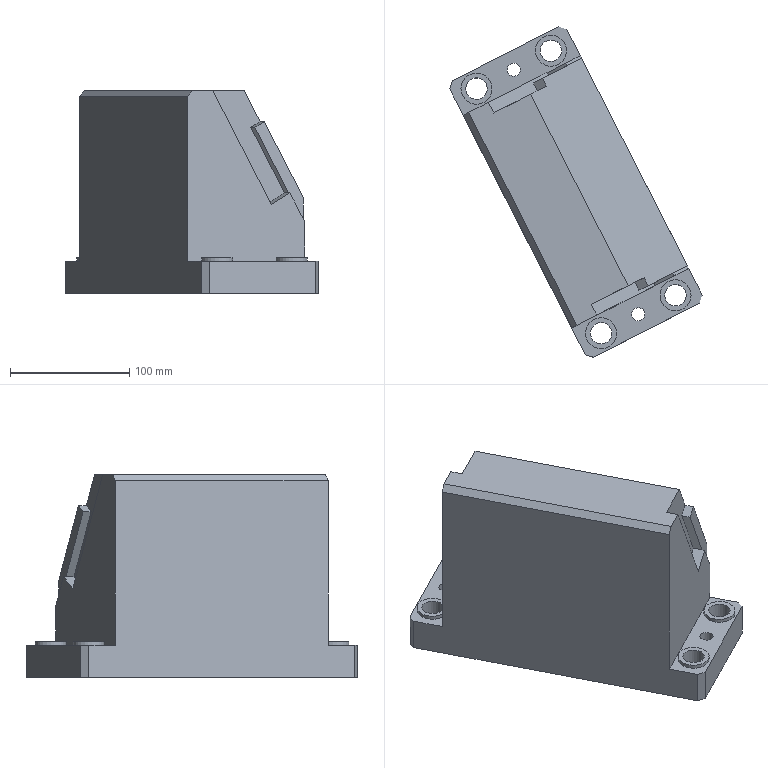Part | NX | features solid 2 | 1 solid | 46 faces | box 211.508 x 277.061 x 170 mm | volume 3366585 mm3 | plane 36 | cylinder 10 | commonest cylinder face diameters 18 x4 26 x4 11 x2
STEP:
#1=CARTESIAN_POINT('',(-1562.486,-605.331,7.));
#2=VERTEX_POINT('',#1);
#3=CARTESIAN_POINT('',(-1574.069,-611.233,7.));
#4=DIRECTION('',(0.,0.,-1.));
#5=DIRECTION('',(0.891,0.454,0.));
#6=AXIS2_PLACEMENT_3D('',#3,#4,#5);
#7=CIRCLE('',#6,13.);
#8=EDGE_CURVE('',#2,#2,#7,.T.);
#9=ORIENTED_EDGE('',*,*,#8,.T.);
#10=EDGE_LOOP('',(#9));
#11=FACE_BOUND('',#10,.T.);
#12=CARTESIAN_POINT('',(-1624.856,-637.11,7.));
#13=VERTEX_POINT('',#12);
#14=CARTESIAN_POINT('',(-1636.44,-643.012,7.));
#15=DIRECTION('',(0.,0.,-1.));
#16=DIRECTION('',(0.891,0.454,0.));
#17=AXIS2_PLACEMENT_3D('',#14,#15,#16);
#18=CIRCLE('',#17,13.);
#19=EDGE_CURVE('',#13,#13,#18,.T.);
#20=ORIENTED_EDGE('',*,*,#19,.T.);
#21=EDGE_LOOP('',(#20));
#22=FACE_BOUND('',#21,.T.);
#23=CARTESIAN_POINT('',(-1600.354,-624.626,7.));
#24=VERTEX_POINT('',#23);
#25=CARTESIAN_POINT('',(-1605.254,-627.122,7.));
#26=DIRECTION('',(0.,0.,-1.));
#27=DIRECTION('',(0.891,0.454,0.));
#28=AXIS2_PLACEMENT_3D('',#25,#26,#27);
#29=CIRCLE('',#28,5.5);
#30=EDGE_CURVE('',#24,#24,#29,.T.);
#31=ORIENTED_EDGE('',*,*,#30,.T.);
#32=EDGE_LOOP('',(#31));
#33=FACE_BOUND('',#32,.T.);
#34=CARTESIAN_POINT('',(-1551.709,-611.063,7.));
#35=VERTEX_POINT('',#34);
#36=CARTESIAN_POINT('',(-1563.059,-588.788,7.));
#37=VERTEX_POINT('',#36);
#38=CARTESIAN_POINT('',(-1563.059,-588.788,7.));
#39=DIRECTION('',(0.454,-0.891,0.));
#40=VECTOR('',#39,1000.);
#41=LINE('',#38,#40);
#42=EDGE_CURVE('',#35,#37,#41,.F.);
#43=ORIENTED_EDGE('',*,*,#42,.T.);
#44=CARTESIAN_POINT('',(-1661.07,-638.727,7.));
#45=VERTEX_POINT('',#44);
#46=CARTESIAN_POINT('',(-1733.241,-675.5,7.));
#47=DIRECTION('',(-0.891,-0.454,0.));
#48=VECTOR('',#47,1000.);
#49=LINE('',#46,#48);
#50=EDGE_CURVE('',#37,#45,#49,.T.);
#51=ORIENTED_EDGE('',*,*,#50,.T.);
#52=CARTESIAN_POINT('',(-1649.72,-661.002,7.));
#53=VERTEX_POINT('',#52);
#54=CARTESIAN_POINT('',(-1661.07,-638.727,7.));
#55=DIRECTION('',(0.454,-0.891,0.));
#56=VECTOR('',#55,1000.);
#57=LINE('',#54,#56);
#58=EDGE_CURVE('',#53,#45,#57,.F.);
#59=ORIENTED_EDGE('',*,*,#58,.F.);
#60=CARTESIAN_POINT('',(-1642.995,-663.187,7.));
#61=VERTEX_POINT('',#60);
#62=CARTESIAN_POINT('',(-1649.72,-661.002,7.));
#63=DIRECTION('',(0.9511,-0.309,0.));
#64=VECTOR('',#63,1000.);
#65=LINE('',#62,#64);
#66=EDGE_CURVE('',#53,#61,#65,.T.);
#67=ORIENTED_EDGE('',*,*,#66,.T.);
#68=CARTESIAN_POINT('',(-1553.894,-617.788,7.));
#69=VERTEX_POINT('',#68);
#70=CARTESIAN_POINT('',(-1642.995,-663.187,7.));
#71=DIRECTION('',(0.891,0.454,0.));
#72=VECTOR('',#71,1000.);
#73=LINE('',#70,#72);
#74=EDGE_CURVE('',#61,#69,#73,.T.);
#75=ORIENTED_EDGE('',*,*,#74,.T.);
#76=CARTESIAN_POINT('',(-1551.709,-611.063,7.));
#77=VERTEX_POINT('',#76);
#78=CARTESIAN_POINT('',(-1551.709,-611.063,7.));
#79=DIRECTION('',(-0.309,-0.9511,0.));
#80=VECTOR('',#79,1000.);
#81=LINE('',#78,#80);
#82=EDGE_CURVE('',#77,#69,#81,.T.);
#83=ORIENTED_EDGE('',*,*,#82,.F.);
#84=CARTESIAN_POINT('',(-1552.6,-611.517,7.));
#85=DIRECTION('',(0.891,0.454,0.));
#86=VECTOR('',#85,1000.);
#87=LINE('',#84,#86);
#88=EDGE_CURVE('',#35,#77,#87,.T.);
#89=ORIENTED_EDGE('',*,*,#88,.F.);
#90=EDGE_LOOP('',(#43,#51,#59,#67,#75,#83,#89));
#91=FACE_BOUND('',#90,.T.);
#92=CARTESIAN_POINT('',(-1765.487,-433.795,7.));
#93=DIRECTION('',(0.,0.,1.));
#94=DIRECTION('',(0.891,0.454,0.));
#95=AXIS2_PLACEMENT_3D('',#92,#93,#94);
#96=PLANE('',#95);
#97=ADVANCED_FACE('',(#11,#22,#33,#91),#96,.T.);
#98=CARTESIAN_POINT('',(-1566.05,-607.147,-20.));
#99=VERTEX_POINT('',#98);
#100=CARTESIAN_POINT('',(-1574.069,-611.233,-20.));
#101=DIRECTION('',(0.,0.,-1.));
#102=DIRECTION('',(0.891,0.454,0.));
#103=AXIS2_PLACEMENT_3D('',#100,#101,#102);
#104=CIRCLE('',#103,9.);
#105=EDGE_CURVE('',#99,#99,#104,.T.);
#106=ORIENTED_EDGE('',*,*,#105,.F.);
#107=EDGE_LOOP('',(#106));
#108=FACE_BOUND('',#107,.T.);
#109=CARTESIAN_POINT('',(-1600.354,-624.626,-20.));
#110=VERTEX_POINT('',#109);
#111=CARTESIAN_POINT('',(-1605.254,-627.122,-20.));
#112=DIRECTION('',(0.,0.,-1.));
#113=DIRECTION('',(0.891,0.454,0.));
#114=AXIS2_PLACEMENT_3D('',#111,#112,#113);
#115=CIRCLE('',#114,5.5);
#116=EDGE_CURVE('',#110,#110,#115,.T.);
#117=ORIENTED_EDGE('',*,*,#116,.F.);
#118=EDGE_LOOP('',(#117));
#119=FACE_BOUND('',#118,.T.);
#120=CARTESIAN_POINT('',(-1628.42,-638.926,-20.));
#121=VERTEX_POINT('',#120);
#122=CARTESIAN_POINT('',(-1636.44,-643.012,-20.));
#123=DIRECTION('',(0.,0.,-1.));
#124=DIRECTION('',(0.891,0.454,0.));
#125=AXIS2_PLACEMENT_3D('',#122,#123,#124);
#126=CIRCLE('',#125,9.);
#127=EDGE_CURVE('',#121,#121,#126,.T.);
#128=ORIENTED_EDGE('',*,*,#127,.F.);
#129=EDGE_LOOP('',(#128));
#130=FACE_BOUND('',#129,.T.);
#131=CARTESIAN_POINT('',(-1670.468,-402.215,-20.));
#132=VERTEX_POINT('',#131);
#133=CARTESIAN_POINT('',(-1678.487,-406.301,-20.));
#134=DIRECTION('',(0.,0.,-1.));
#135=DIRECTION('',(0.891,0.454,0.));
#136=AXIS2_PLACEMENT_3D('',#133,#134,#135);
#137=CIRCLE('',#136,9.);
#138=EDGE_CURVE('',#132,#132,#137,.T.);
#139=ORIENTED_EDGE('',*,*,#138,.F.);
#140=EDGE_LOOP('',(#139));
#141=FACE_BOUND('',#140,.T.);
#142=CARTESIAN_POINT('',(-1704.772,-419.694,-20.));
#143=VERTEX_POINT('',#142);
#144=CARTESIAN_POINT('',(-1709.672,-422.191,-20.));
#145=DIRECTION('',(0.,0.,-1.));
#146=DIRECTION('',(0.891,0.454,0.));
#147=AXIS2_PLACEMENT_3D('',#144,#145,#146);
#148=CIRCLE('',#147,5.5);
#149=EDGE_CURVE('',#143,#143,#148,.T.);
#150=ORIENTED_EDGE('',*,*,#149,.F.);
#151=EDGE_LOOP('',(#150));
#152=FACE_BOUND('',#151,.T.);
#153=CARTESIAN_POINT('',(-1732.838,-433.995,-20.));
#154=VERTEX_POINT('',#153);
#155=CARTESIAN_POINT('',(-1740.857,-438.081,-20.));
#156=DIRECTION('',(0.,0.,-1.));
#157=DIRECTION('',(0.891,0.454,0.));
#158=AXIS2_PLACEMENT_3D('',#155,#156,#157);
#159=CIRCLE('',#158,9.);
#160=EDGE_CURVE('',#154,#154,#159,.T.);
#161=ORIENTED_EDGE('',*,*,#160,.F.);
#162=EDGE_LOOP('',(#161));
#163=FACE_BOUND('',#162,.T.);
#164=CARTESIAN_POINT('',(-1551.709,-611.063,-20.));
#165=VERTEX_POINT('',#164);
#166=CARTESIAN_POINT('',(-1551.709,-611.063,-20.));
#167=VERTEX_POINT('',#166);
#168=CARTESIAN_POINT('',(-1552.6,-611.517,-20.));
#169=DIRECTION('',(0.891,0.454,0.));
#170=VECTOR('',#169,1000.);
#171=LINE('',#168,#170);
#172=EDGE_CURVE('',#165,#167,#171,.T.);
#173=ORIENTED_EDGE('',*,*,#172,.T.);
#174=CARTESIAN_POINT('',(-1553.894,-617.788,-20.));
#175=VERTEX_POINT('',#174);
#176=CARTESIAN_POINT('',(-1551.709,-611.063,-20.));
#177=DIRECTION('',(-0.309,-0.9511,0.));
#178=VECTOR('',#177,1000.);
#179=LINE('',#176,#178);
#180=EDGE_CURVE('',#167,#175,#179,.T.);
#181=ORIENTED_EDGE('',*,*,#180,.T.);
#182=CARTESIAN_POINT('',(-1642.995,-663.187,-20.));
#183=VERTEX_POINT('',#182);
#184=CARTESIAN_POINT('',(-1642.995,-663.187,-20.));
#185=DIRECTION('',(0.891,0.454,0.));
#186=VECTOR('',#185,1000.);
#187=LINE('',#184,#186);
#188=EDGE_CURVE('',#183,#175,#187,.T.);
#189=ORIENTED_EDGE('',*,*,#188,.F.);
#190=CARTESIAN_POINT('',(-1649.72,-661.002,-20.));
#191=VERTEX_POINT('',#190);
#192=CARTESIAN_POINT('',(-1649.72,-661.002,-20.));
#193=DIRECTION('',(0.9511,-0.309,0.));
#194=VECTOR('',#193,1000.);
#195=LINE('',#192,#194);
#196=EDGE_CURVE('',#191,#183,#195,.T.);
#197=ORIENTED_EDGE('',*,*,#196,.F.);
#198=CARTESIAN_POINT('',(-1763.218,-438.251,-20.));
#199=VERTEX_POINT('',#198);
#200=CARTESIAN_POINT('',(-1661.07,-638.727,-20.));
#201=DIRECTION('',(0.454,-0.891,0.));
#202=VECTOR('',#201,1000.);
#203=LINE('',#200,#202);
#204=EDGE_CURVE('',#191,#199,#203,.F.);
#205=ORIENTED_EDGE('',*,*,#204,.T.);
#206=CARTESIAN_POINT('',(-1761.032,-431.525,-20.));
#207=VERTEX_POINT('',#206);
#208=CARTESIAN_POINT('',(-1761.032,-431.525,-20.));
#209=DIRECTION('',(-0.309,-0.9511,0.));
#210=VECTOR('',#209,1000.);
#211=LINE('',#208,#210);
#212=EDGE_CURVE('',#207,#199,#211,.T.);
#213=ORIENTED_EDGE('',*,*,#212,.F.);
#214=CARTESIAN_POINT('',(-1671.932,-386.126,-20.));
#215=VERTEX_POINT('',#214);
#216=CARTESIAN_POINT('',(-1761.032,-431.525,-20.));
#217=DIRECTION('',(0.891,0.454,0.));
#218=VECTOR('',#217,1000.);
#219=LINE('',#216,#218);
#220=EDGE_CURVE('',#207,#215,#219,.T.);
#221=ORIENTED_EDGE('',*,*,#220,.T.);
#222=CARTESIAN_POINT('',(-1665.207,-388.311,-20.));
#223=VERTEX_POINT('',#222);
#224=CARTESIAN_POINT('',(-1671.932,-386.126,-20.));
#225=DIRECTION('',(0.9511,-0.309,0.));
#226=VECTOR('',#225,1000.);
#227=LINE('',#224,#226);
#228=EDGE_CURVE('',#215,#223,#227,.T.);
#229=ORIENTED_EDGE('',*,*,#228,.T.);
#230=CARTESIAN_POINT('',(-1665.207,-388.312,-20.));
#231=VERTEX_POINT('',#230);
#232=CARTESIAN_POINT('',(-1666.098,-388.765,-20.));
#233=DIRECTION('',(0.891,0.454,0.));
#234=VECTOR('',#233,1000.);
#235=LINE('',#232,#234);
#236=EDGE_CURVE('',#231,#223,#235,.T.);
#237=ORIENTED_EDGE('',*,*,#236,.F.);
#238=CARTESIAN_POINT('',(-1563.059,-588.788,-20.));
#239=DIRECTION('',(-0.454,0.891,0.));
#240=VECTOR('',#239,1000.);
#241=LINE('',#238,#240);
#242=EDGE_CURVE('',#165,#231,#241,.T.);
#243=ORIENTED_EDGE('',*,*,#242,.F.);
#244=EDGE_LOOP('',(#173,#181,#189,#197,#205,#213,#221,#229,#237,#243));
#245=FACE_BOUND('',#244,.T.);
#246=CARTESIAN_POINT('',(-1563.059,-588.788,-20.));
#247=DIRECTION('',(0.,0.,1.));
#248=DIRECTION('',(0.891,0.454,0.));
#249=AXIS2_PLACEMENT_3D('',#246,#247,#248);
#250=PLANE('',#249);
#251=ADVANCED_FACE('',(#108,#119,#130,#141,#152,#163,#245),#250,.F.);
#252=CARTESIAN_POINT('',(-1613.811,-603.424,150.));
#253=VERTEX_POINT('',#252);
#254=CARTESIAN_POINT('',(-1695.53,-443.043,150.));
#255=VERTEX_POINT('',#254);
#256=CARTESIAN_POINT('',(-1610.406,-610.107,150.));
#257=DIRECTION('',(-0.454,0.891,0.));
#258=VECTOR('',#257,1000.);
#259=LINE('',#256,#258);
#260=EDGE_CURVE('',#253,#255,#259,.T.);
#261=ORIENTED_EDGE('',*,*,#260,.T.);
#262=CARTESIAN_POINT('',(-1726.395,-458.77,150.));
#263=VERTEX_POINT('',#262);
#264=CARTESIAN_POINT('',(-1705.818,-448.285,150.));
#265=DIRECTION('',(0.891,0.454,0.));
#266=VECTOR('',#265,1000.);
#267=LINE('',#264,#266);
#268=EDGE_CURVE('',#263,#255,#267,.T.);
#269=ORIENTED_EDGE('',*,*,#268,.F.);
#270=CARTESIAN_POINT('',(-1730.935,-449.86,150.));
#271=VERTEX_POINT('',#270);
#272=CARTESIAN_POINT('',(-1640.137,-628.061,150.));
#273=DIRECTION('',(0.454,-0.891,0.));
#274=VECTOR('',#273,1000.);
#275=LINE('',#272,#274);
#276=EDGE_CURVE('',#271,#263,#275,.T.);
#277=ORIENTED_EDGE('',*,*,#276,.F.);
#278=CARTESIAN_POINT('',(-1747.413,-458.256,150.));
#279=VERTEX_POINT('',#278);
#280=CARTESIAN_POINT('',(-1710.358,-439.375,150.));
#281=DIRECTION('',(-0.891,-0.454,0.));
#282=VECTOR('',#281,1000.);
#283=LINE('',#280,#282);
#284=EDGE_CURVE('',#271,#279,#283,.T.);
#285=ORIENTED_EDGE('',*,*,#284,.T.);
#286=CARTESIAN_POINT('',(-1656.615,-636.457,150.));
#287=VERTEX_POINT('',#286);
#288=CARTESIAN_POINT('',(-1656.615,-636.457,150.));
#289=DIRECTION('',(-0.454,0.891,0.));
#290=VECTOR('',#289,1000.);
#291=LINE('',#288,#290);
#292=EDGE_CURVE('',#287,#279,#291,.T.);
#293=ORIENTED_EDGE('',*,*,#292,.F.);
#294=CARTESIAN_POINT('',(-1640.137,-628.061,150.));
#295=VERTEX_POINT('',#294);
#296=CARTESIAN_POINT('',(-1619.56,-617.577,150.));
#297=DIRECTION('',(-0.891,-0.454,0.));
#298=VECTOR('',#297,1000.);
#299=LINE('',#296,#298);
#300=EDGE_CURVE('',#295,#287,#299,.T.);
#301=ORIENTED_EDGE('',*,*,#300,.F.);
#302=CARTESIAN_POINT('',(-1644.677,-619.151,150.));
#303=VERTEX_POINT('',#302);
#304=CARTESIAN_POINT('',(-1640.137,-628.061,150.));
#305=DIRECTION('',(-0.454,0.891,0.));
#306=VECTOR('',#305,1000.);
#307=LINE('',#304,#306);
#308=EDGE_CURVE('',#295,#303,#307,.T.);
#309=ORIENTED_EDGE('',*,*,#308,.T.);
#310=CARTESIAN_POINT('',(-1624.1,-608.667,150.));
#311=DIRECTION('',(0.891,0.454,0.));
#312=VECTOR('',#311,1000.);
#313=LINE('',#310,#312);
#314=EDGE_CURVE('',#303,#253,#313,.T.);
#315=ORIENTED_EDGE('',*,*,#314,.T.);
#316=EDGE_LOOP('',(#261,#269,#277,#285,#293,#301,#309,#315));
#317=FACE_BOUND('',#316,.T.);
#318=CARTESIAN_POINT('',(-1619.56,-617.577,150.));
#319=DIRECTION('',(0.,0.,1.));
#320=DIRECTION('',(0.891,0.454,0.));
#321=AXIS2_PLACEMENT_3D('',#318,#319,#320);
#322=PLANE('',#321);
#323=ADVANCED_FACE('',(#317),#322,.T.);
#324=CARTESIAN_POINT('',(-1597.019,-603.285,123.975));
#325=VERTEX_POINT('',#324);
#326=CARTESIAN_POINT('',(-1564.194,-586.561,60.167));
#327=VERTEX_POINT('',#326);
#328=CARTESIAN_POINT('',(-1610.406,-610.107,150.));
#329=DIRECTION('',(0.4455,0.227,-0.866));
#330=VECTOR('',#329,1000.);
#331=LINE('',#328,#330);
#332=EDGE_CURVE('',#325,#327,#331,.T.);
#333=ORIENTED_EDGE('',*,*,#332,.T.);
#334=CARTESIAN_POINT('',(-1652.722,-412.814,60.167));
#335=VERTEX_POINT('',#334);
#336=CARTESIAN_POINT('',(-1564.194,-586.561,60.167));
#337=DIRECTION('',(-0.454,0.891,0.));
#338=VECTOR('',#337,1000.);
#339=LINE('',#336,#338);
#340=EDGE_CURVE('',#327,#335,#339,.T.);
#341=ORIENTED_EDGE('',*,*,#340,.T.);
#342=CARTESIAN_POINT('',(-1685.547,-429.539,123.975));
#343=VERTEX_POINT('',#342);
#344=CARTESIAN_POINT('',(-1698.935,-436.361,150.));
#345=DIRECTION('',(0.4455,0.227,-0.866));
#346=VECTOR('',#345,1000.);
#347=LINE('',#344,#346);
#348=EDGE_CURVE('',#343,#335,#347,.T.);
#349=ORIENTED_EDGE('',*,*,#348,.F.);
#350=CARTESIAN_POINT('',(-1682.142,-436.222,123.975));
#351=VERTEX_POINT('',#350);
#352=CARTESIAN_POINT('',(-1597.019,-603.285,123.975));
#353=DIRECTION('',(0.454,-0.891,0.));
#354=VECTOR('',#353,1000.);
#355=LINE('',#352,#354);
#356=EDGE_CURVE('',#343,#351,#355,.T.);
#357=ORIENTED_EDGE('',*,*,#356,.T.);
#358=CARTESIAN_POINT('',(-1695.53,-443.043,150.));
#359=DIRECTION('',(0.4455,0.227,-0.866));
#360=VECTOR('',#359,1000.);
#361=LINE('',#358,#360);
#362=EDGE_CURVE('',#255,#351,#361,.T.);
#363=ORIENTED_EDGE('',*,*,#362,.F.);
#364=ORIENTED_EDGE('',*,*,#260,.F.);
#365=CARTESIAN_POINT('',(-1600.423,-596.603,123.975));
#366=VERTEX_POINT('',#365);
#367=CARTESIAN_POINT('',(-1613.811,-603.424,150.));
#368=DIRECTION('',(0.4455,0.227,-0.866));
#369=VECTOR('',#368,1000.);
#370=LINE('',#367,#369);
#371=EDGE_CURVE('',#253,#366,#370,.T.);
#372=ORIENTED_EDGE('',*,*,#371,.T.);
#373=CARTESIAN_POINT('',(-1597.019,-603.285,123.975));
#374=DIRECTION('',(0.454,-0.891,0.));
#375=VECTOR('',#374,1000.);
#376=LINE('',#373,#375);
#377=EDGE_CURVE('',#325,#366,#376,.F.);
#378=ORIENTED_EDGE('',*,*,#377,.F.);
#379=EDGE_LOOP('',(#333,#341,#349,#357,#363,#364,#372,#378));
#380=FACE_BOUND('',#379,.T.);
#381=CARTESIAN_POINT('',(-1610.406,-610.107,150.));
#382=DIRECTION('',(-0.7716,-0.3932,-0.5));
#383=DIRECTION('',(-0.4455,-0.227,0.866));
#384=AXIS2_PLACEMENT_3D('',#381,#382,#383);
#385=PLANE('',#384);
#386=ADVANCED_FACE('',(#380),#385,.F.);
#387=CARTESIAN_POINT('',(-1693.263,-433.471,118.975));
#388=VERTEX_POINT('',#387);
#389=CARTESIAN_POINT('',(-1693.263,-433.471,118.975));
#390=DIRECTION('',(0.7716,0.3932,0.5));
#391=VECTOR('',#390,1000.);
#392=LINE('',#389,#391);
#393=EDGE_CURVE('',#388,#343,#392,.T.);
#394=ORIENTED_EDGE('',*,*,#393,.T.);
#395=ORIENTED_EDGE('',*,*,#348,.T.);
#396=CARTESIAN_POINT('',(-1652.722,-412.814,40.167));
#397=VERTEX_POINT('',#396);
#398=CARTESIAN_POINT('',(-1652.722,-412.814,60.167));
#399=DIRECTION('',(0.,0.,-1.));
#400=VECTOR('',#399,1000.);
#401=LINE('',#398,#400);
#402=EDGE_CURVE('',#335,#397,#401,.T.);
#403=ORIENTED_EDGE('',*,*,#402,.T.);
#404=CARTESIAN_POINT('',(-1665.196,-419.17,64.415));
#405=VERTEX_POINT('',#404);
#406=CARTESIAN_POINT('',(-1679.452,-426.434,92.128));
#407=DIRECTION('',(-0.4455,-0.227,0.866));
#408=VECTOR('',#407,1000.);
#409=LINE('',#406,#408);
#410=EDGE_CURVE('',#397,#405,#409,.T.);
#411=ORIENTED_EDGE('',*,*,#410,.T.);
#412=CARTESIAN_POINT('',(-1679.452,-426.434,92.128));
#413=DIRECTION('',(-0.4455,-0.227,0.866));
#414=VECTOR('',#413,1000.);
#415=LINE('',#412,#414);
#416=EDGE_CURVE('',#405,#388,#415,.T.);
#417=ORIENTED_EDGE('',*,*,#416,.T.);
#418=EDGE_LOOP('',(#394,#395,#403,#411,#417));
#419=FACE_BOUND('',#418,.T.);
#420=CARTESIAN_POINT('',(-1652.722,-412.814,150.));
#421=DIRECTION('',(0.454,-0.891,0.));
#422=DIRECTION('',(-0.891,-0.454,0.));
#423=AXIS2_PLACEMENT_3D('',#420,#421,#422);
#424=PLANE('',#423);
#425=ADVANCED_FACE('',(#419),#424,.F.);
#426=CARTESIAN_POINT('',(-1689.858,-440.153,118.975));
#427=VERTEX_POINT('',#426);
#428=CARTESIAN_POINT('',(-1693.263,-433.471,118.975));
#429=DIRECTION('',(0.454,-0.891,0.));
#430=VECTOR('',#429,1000.);
#431=LINE('',#428,#430);
#432=EDGE_CURVE('',#427,#388,#431,.F.);
#433=ORIENTED_EDGE('',*,*,#432,.T.);
#434=ORIENTED_EDGE('',*,*,#416,.F.);
#435=CARTESIAN_POINT('',(-1661.791,-425.853,64.415));
#436=VERTEX_POINT('',#435);
#437=CARTESIAN_POINT('',(-1662.699,-424.071,64.415));
#438=DIRECTION('',(-0.454,0.891,0.));
#439=VECTOR('',#438,1000.);
#440=LINE('',#437,#439);
#441=EDGE_CURVE('',#436,#405,#440,.T.);
#442=ORIENTED_EDGE('',*,*,#441,.F.);
#443=CARTESIAN_POINT('',(-1738.418,-464.896,213.372));
#444=DIRECTION('',(-0.4455,-0.227,0.866));
#445=VECTOR('',#444,1000.);
#446=LINE('',#443,#445);
#447=EDGE_CURVE('',#427,#436,#446,.F.);
#448=ORIENTED_EDGE('',*,*,#447,.F.);
#449=EDGE_LOOP('',(#433,#434,#442,#448));
#450=FACE_BOUND('',#449,.T.);
#451=CARTESIAN_POINT('',(-1676.955,-431.334,92.128));
#452=DIRECTION('',(0.7716,0.3932,0.5));
#453=DIRECTION('',(0.4455,0.227,-0.866));
#454=AXIS2_PLACEMENT_3D('',#451,#452,#453);
#455=PLANE('',#454);
#456=ADVANCED_FACE('',(#450),#455,.F.);
#457=CARTESIAN_POINT('',(-1681.764,-424.806,54.415));
#458=VERTEX_POINT('',#457);
#459=CARTESIAN_POINT('',(-1666.331,-416.943,64.415));
#460=VERTEX_POINT('',#459);
#461=CARTESIAN_POINT('',(-1681.764,-424.806,54.415));
#462=DIRECTION('',(0.7716,0.3932,0.5));
#463=VECTOR('',#462,1000.);
#464=LINE('',#461,#463);
#465=EDGE_CURVE('',#458,#460,#464,.T.);
#466=ORIENTED_EDGE('',*,*,#465,.T.);
#467=CARTESIAN_POINT('',(-1653.857,-410.587,40.167));
#468=VERTEX_POINT('',#467);
#469=CARTESIAN_POINT('',(-1705.598,-436.95,140.747));
#470=DIRECTION('',(-0.4455,-0.227,0.866));
#471=VECTOR('',#470,1000.);
#472=LINE('',#469,#471);
#473=EDGE_CURVE('',#468,#460,#472,.T.);
#474=ORIENTED_EDGE('',*,*,#473,.F.);
#475=CARTESIAN_POINT('',(-1653.857,-410.587,7.));
#476=VERTEX_POINT('',#475);
#477=CARTESIAN_POINT('',(-1653.857,-410.587,40.167));
#478=DIRECTION('',(0.,0.,-1.));
#479=VECTOR('',#478,1000.);
#480=LINE('',#477,#479);
#481=EDGE_CURVE('',#468,#476,#480,.T.);
#482=ORIENTED_EDGE('',*,*,#481,.T.);
#483=CARTESIAN_POINT('',(-1751.868,-460.526,7.));
#484=VERTEX_POINT('',#483);
#485=CARTESIAN_POINT('',(-1824.039,-497.299,7.));
#486=DIRECTION('',(-0.891,-0.454,0.));
#487=VECTOR('',#486,1000.);
#488=LINE('',#485,#487);
#489=EDGE_CURVE('',#476,#484,#488,.T.);
#490=ORIENTED_EDGE('',*,*,#489,.T.);
#491=CARTESIAN_POINT('',(-1751.868,-460.526,145.));
#492=VERTEX_POINT('',#491);
#493=CARTESIAN_POINT('',(-1751.868,-460.526,7.));
#494=DIRECTION('',(0.,0.,-1.));
#495=VECTOR('',#494,1000.);
#496=LINE('',#493,#495);
#497=EDGE_CURVE('',#492,#484,#496,.T.);
#498=ORIENTED_EDGE('',*,*,#497,.F.);
#499=CARTESIAN_POINT('',(-1747.413,-458.256,150.));
#500=DIRECTION('',(-0.63,-0.321,-0.7071));
#501=VECTOR('',#500,1000.);
#502=LINE('',#499,#501);
#503=EDGE_CURVE('',#279,#492,#502,.T.);
#504=ORIENTED_EDGE('',*,*,#503,.F.);
#505=ORIENTED_EDGE('',*,*,#284,.F.);
#506=CARTESIAN_POINT('',(-1758.391,-463.849,203.372));
#507=DIRECTION('',(0.4455,0.227,-0.866));
#508=VECTOR('',#507,1000.);
#509=LINE('',#506,#508);
#510=EDGE_CURVE('',#271,#458,#509,.T.);
#511=ORIENTED_EDGE('',*,*,#510,.T.);
#512=EDGE_LOOP('',(#466,#474,#482,#490,#498,#504,#505,#511));
#513=FACE_BOUND('',#512,.T.);
#514=CARTESIAN_POINT('',(-1824.039,-497.299,64.));
#515=DIRECTION('',(-0.454,0.891,0.));
#516=DIRECTION('',(0.,0.,-1.));
#517=AXIS2_PLACEMENT_3D('',#514,#515,#516);
#518=PLANE('',#517);
#519=ADVANCED_FACE('',(#513),#518,.T.);
#520=ORIENTED_EDGE('',*,*,#410,.F.);
#521=CARTESIAN_POINT('',(-1650.225,-417.715,40.167));
#522=DIRECTION('',(-0.454,0.891,0.));
#523=VECTOR('',#522,1000.);
#524=LINE('',#521,#523);
#525=EDGE_CURVE('',#397,#468,#524,.T.);
#526=ORIENTED_EDGE('',*,*,#525,.T.);
#527=ORIENTED_EDGE('',*,*,#473,.T.);
#528=CARTESIAN_POINT('',(-1662.699,-424.071,64.415));
#529=DIRECTION('',(-0.454,0.891,0.));
#530=VECTOR('',#529,1000.);
#531=LINE('',#528,#530);
#532=EDGE_CURVE('',#405,#460,#531,.T.);
#533=ORIENTED_EDGE('',*,*,#532,.F.);
#534=EDGE_LOOP('',(#520,#526,#527,#533));
#535=FACE_BOUND('',#534,.T.);
#536=CARTESIAN_POINT('',(-1676.955,-431.334,92.128));
#537=DIRECTION('',(0.7716,0.3932,0.5));
#538=DIRECTION('',(0.4455,0.227,-0.866));
#539=AXIS2_PLACEMENT_3D('',#536,#537,#538);
#540=PLANE('',#539);
#541=ADVANCED_FACE('',(#535),#540,.T.);
#542=ORIENTED_EDGE('',*,*,#300,.T.);
#543=CARTESIAN_POINT('',(-1661.07,-638.727,145.));
#544=VERTEX_POINT('',#543);
#545=CARTESIAN_POINT('',(-1656.615,-636.457,150.));
#546=DIRECTION('',(-0.63,-0.321,-0.7071));
#547=VECTOR('',#546,1000.);
#548=LINE('',#545,#547);
#549=EDGE_CURVE('',#287,#544,#548,.T.);
#550=ORIENTED_EDGE('',*,*,#549,.T.);
#551=CARTESIAN_POINT('',(-1661.07,-638.727,145.));
#552=DIRECTION('',(0.,0.,-1.));
#553=VECTOR('',#552,1000.);
#554=LINE('',#551,#553);
#555=EDGE_CURVE('',#544,#45,#554,.T.);
#556=ORIENTED_EDGE('',*,*,#555,.T.);
#557=ORIENTED_EDGE('',*,*,#50,.F.);
#558=CARTESIAN_POINT('',(-1563.059,-588.788,40.167));
#559=VERTEX_POINT('',#558);
#560=CARTESIAN_POINT('',(-1563.059,-588.788,7.));
#561=DIRECTION('',(0.,0.,-1.));
#562=VECTOR('',#561,1000.);
#563=LINE('',#560,#562);
#564=EDGE_CURVE('',#559,#37,#563,.T.);
#565=ORIENTED_EDGE('',*,*,#564,.F.);
#566=CARTESIAN_POINT('',(-1575.533,-595.144,64.415));
#567=VERTEX_POINT('',#566);
#568=CARTESIAN_POINT('',(-1589.789,-602.408,92.128));
#569=DIRECTION('',(-0.4455,-0.227,0.866));
#570=VECTOR('',#569,1000.);
#571=LINE('',#568,#570);
#572=EDGE_CURVE('',#559,#567,#571,.T.);
#573=ORIENTED_EDGE('',*,*,#572,.T.);
#574=CARTESIAN_POINT('',(-1590.966,-603.007,54.415));
#575=VERTEX_POINT('',#574);
#576=CARTESIAN_POINT('',(-1590.966,-603.007,54.415));
#577=DIRECTION('',(0.7716,0.3932,0.5));
#578=VECTOR('',#577,1000.);
#579=LINE('',#576,#578);
#580=EDGE_CURVE('',#575,#567,#579,.T.);
#581=ORIENTED_EDGE('',*,*,#580,.F.);
#582=CARTESIAN_POINT('',(-1667.592,-642.05,203.372));
#583=DIRECTION('',(0.4455,0.227,-0.866));
#584=VECTOR('',#583,1000.);
#585=LINE('',#582,#584);
#586=EDGE_CURVE('',#295,#575,#585,.T.);
#587=ORIENTED_EDGE('',*,*,#586,.F.);
#588=EDGE_LOOP('',(#542,#550,#556,#557,#565,#573,#581,#587));
#589=FACE_BOUND('',#588,.T.);
#590=CARTESIAN_POINT('',(-1733.241,-675.5,64.));
#591=DIRECTION('',(-0.454,0.891,0.));
#592=DIRECTION('',(0.,0.,-1.));
#593=AXIS2_PLACEMENT_3D('',#590,#591,#592);
#594=PLANE('',#593);
#595=ADVANCED_FACE('',(#589),#594,.F.);
#596=ORIENTED_EDGE('',*,*,#503,.T.);
#597=CARTESIAN_POINT('',(-1661.07,-638.727,145.));
#598=DIRECTION('',(-0.454,0.891,0.));
#599=VECTOR('',#598,1000.);
#600=LINE('',#597,#599);
#601=EDGE_CURVE('',#544,#492,#600,.T.);
#602=ORIENTED_EDGE('',*,*,#601,.F.);
#603=ORIENTED_EDGE('',*,*,#549,.F.);
#604=ORIENTED_EDGE('',*,*,#292,.T.);
#605=EDGE_LOOP('',(#596,#602,#603,#604));
#606=FACE_BOUND('',#605,.T.);
#607=CARTESIAN_POINT('',(-1656.615,-636.457,150.));
#608=DIRECTION('',(-0.63,-0.321,0.7071));
#609=DIRECTION('',(0.63,0.321,0.7071));
#610=AXIS2_PLACEMENT_3D('',#607,#608,#609);
#611=PLANE('',#610);
#612=ADVANCED_FACE('',(#606),#611,.T.);
#613=ORIENTED_EDGE('',*,*,#555,.F.);
#614=ORIENTED_EDGE('',*,*,#601,.T.);
#615=ORIENTED_EDGE('',*,*,#497,.T.);
#616=CARTESIAN_POINT('',(-1763.218,-438.251,7.));
#617=VERTEX_POINT('',#616);
#618=CARTESIAN_POINT('',(-1661.07,-638.727,7.));
#619=DIRECTION('',(0.454,-0.891,0.));
#620=VECTOR('',#619,1000.);
#621=LINE('',#618,#620);
#622=EDGE_CURVE('',#484,#617,#621,.F.);
#623=ORIENTED_EDGE('',*,*,#622,.T.);
#624=CARTESIAN_POINT('',(-1763.218,-438.251,7.));
#625=DIRECTION('',(0.,0.,1.));
#626=VECTOR('',#625,1000.);
#627=LINE('',#624,#626);
#628=EDGE_CURVE('',#617,#199,#627,.F.);
#629=ORIENTED_EDGE('',*,*,#628,.T.);
#630=ORIENTED_EDGE('',*,*,#204,.F.);
#631=CARTESIAN_POINT('',(-1649.72,-661.002,7.));
#632=DIRECTION('',(0.,0.,1.));
#633=VECTOR('',#632,1000.);
#634=LINE('',#631,#633);
#635=EDGE_CURVE('',#53,#191,#634,.F.);
#636=ORIENTED_EDGE('',*,*,#635,.F.);
#637=ORIENTED_EDGE('',*,*,#58,.T.);
#638=EDGE_LOOP('',(#613,#614,#615,#623,#629,#630,#636,#637));
#639=FACE_BOUND('',#638,.T.);
#640=CARTESIAN_POINT('',(-1661.07,-638.727,7.));
#641=DIRECTION('',(-0.891,-0.454,0.));
#642=DIRECTION('',(0.,0.,1.));
#643=AXIS2_PLACEMENT_3D('',#640,#641,#642);
#644=PLANE('',#643);
#645=ADVANCED_FACE('',(#639),#644,.T.);
#646=ORIENTED_EDGE('',*,*,#481,.F.);
#647=ORIENTED_EDGE('',*,*,#525,.F.);
#648=ORIENTED_EDGE('',*,*,#402,.F.);
#649=ORIENTED_EDGE('',*,*,#340,.F.);
#650=CARTESIAN_POINT('',(-1564.194,-586.561,40.167));
#651=VERTEX_POINT('',#650);
#652=CARTESIAN_POINT('',(-1564.194,-586.561,60.167));
#653=DIRECTION('',(0.,0.,-1.));
#654=VECTOR('',#653,1000.);
#655=LINE('',#652,#654);
#656=EDGE_CURVE('',#327,#651,#655,.T.);
#657=ORIENTED_EDGE('',*,*,#656,.T.);
#658=CARTESIAN_POINT('',(-1563.059,-588.788,40.167));
#659=DIRECTION('',(-0.454,0.891,0.));
#660=VECTOR('',#659,1000.);
#661=LINE('',#658,#660);
#662=EDGE_CURVE('',#559,#651,#661,.T.);
#663=ORIENTED_EDGE('',*,*,#662,.F.);
#664=ORIENTED_EDGE('',*,*,#564,.T.);
#665=ORIENTED_EDGE('',*,*,#42,.F.);
#666=CARTESIAN_POINT('',(-1551.709,-611.063,7.));
#667=DIRECTION('',(0.,0.,-1.));
#668=VECTOR('',#667,1000.);
#669=LINE('',#666,#668);
#670=EDGE_CURVE('',#35,#165,#669,.T.);
#671=ORIENTED_EDGE('',*,*,#670,.T.);
#672=ORIENTED_EDGE('',*,*,#242,.T.);
#673=CARTESIAN_POINT('',(-1665.207,-388.312,7.));
#674=VERTEX_POINT('',#673);
#675=CARTESIAN_POINT('',(-1665.207,-388.312,7.));
#676=DIRECTION('',(0.,0.,-1.));
#677=VECTOR('',#676,1000.);
#678=LINE('',#675,#677);
#679=EDGE_CURVE('',#674,#231,#678,.T.);
#680=ORIENTED_EDGE('',*,*,#679,.F.);
#681=CARTESIAN_POINT('',(-1563.059,-588.788,7.));
#682=DIRECTION('',(0.454,-0.891,0.));
#683=VECTOR('',#682,1000.);
#684=LINE('',#681,#683);
#685=EDGE_CURVE('',#476,#674,#684,.F.);
#686=ORIENTED_EDGE('',*,*,#685,.F.);
#687=EDGE_LOOP('',(#646,#647,#648,#649,#657,#663,#664,#665,#671,#672,#680,#686));
#688=FACE_BOUND('',#687,.T.);
#689=CARTESIAN_POINT('',(-1563.059,-588.788,40.167));
#690=DIRECTION('',(-0.891,-0.454,0.));
#691=DIRECTION('',(0.,0.,1.));
#692=AXIS2_PLACEMENT_3D('',#689,#690,#691);
#693=PLANE('',#692);
#694=ADVANCED_FACE('',(#688),#693,.F.);
#695=CARTESIAN_POINT('',(-1576.668,-592.916,64.415));
#696=VERTEX_POINT('',#695);
#697=CARTESIAN_POINT('',(-1579.165,-588.016,64.415));
#698=DIRECTION('',(-0.454,0.891,0.));
#699=VECTOR('',#698,1000.);
#700=LINE('',#697,#699);
#701=EDGE_CURVE('',#696,#567,#700,.F.);
#702=ORIENTED_EDGE('',*,*,#701,.T.);
#703=ORIENTED_EDGE('',*,*,#572,.F.);
#704=ORIENTED_EDGE('',*,*,#662,.T.);
#705=CARTESIAN_POINT('',(-1590.924,-600.18,92.128));
#706=DIRECTION('',(0.4455,0.227,-0.866));
#707=VECTOR('',#706,1000.);
#708=LINE('',#705,#707);
#709=EDGE_CURVE('',#651,#696,#708,.F.);
#710=ORIENTED_EDGE('',*,*,#709,.T.);
#711=EDGE_LOOP('',(#702,#703,#704,#710));
#712=FACE_BOUND('',#711,.T.);
#713=CARTESIAN_POINT('',(-1593.421,-595.28,92.128));
#714=DIRECTION('',(-0.7716,-0.3932,-0.5));
#715=DIRECTION('',(-0.4455,-0.227,0.866));
#716=AXIS2_PLACEMENT_3D('',#713,#714,#715);
#717=PLANE('',#716);
#718=ADVANCED_FACE('',(#712),#717,.F.);
#719=CARTESIAN_POINT('',(-1604.735,-607.217,118.975));
#720=VERTEX_POINT('',#719);
#721=CARTESIAN_POINT('',(-1604.735,-607.217,118.975));
#722=DIRECTION('',(0.7716,0.3932,0.5));
#723=VECTOR('',#722,1000.);
#724=LINE('',#721,#723);
#725=EDGE_CURVE('',#720,#325,#724,.T.);
#726=ORIENTED_EDGE('',*,*,#725,.F.);
#727=CARTESIAN_POINT('',(-1606.57,-608.152,122.542));
#728=DIRECTION('',(-0.4455,-0.227,0.866));
#729=VECTOR('',#728,1000.);
#730=LINE('',#727,#729);
#731=EDGE_CURVE('',#696,#720,#730,.T.);
#732=ORIENTED_EDGE('',*,*,#731,.F.);
#733=ORIENTED_EDGE('',*,*,#709,.F.);
#734=ORIENTED_EDGE('',*,*,#656,.F.);
#735=ORIENTED_EDGE('',*,*,#332,.F.);
#736=EDGE_LOOP('',(#726,#732,#733,#734,#735));
#737=FACE_BOUND('',#736,.T.);
#738=CARTESIAN_POINT('',(-1564.194,-586.561,150.));
#739=DIRECTION('',(0.454,-0.891,0.));
#740=DIRECTION('',(-0.891,-0.454,0.));
#741=AXIS2_PLACEMENT_3D('',#738,#739,#740);
#742=PLANE('',#741);
#743=ADVANCED_FACE('',(#737),#742,.T.);
#744=CARTESIAN_POINT('',(-1665.207,-388.311,7.));
#745=VERTEX_POINT('',#744);
#746=CARTESIAN_POINT('',(-1666.098,-388.765,7.));
#747=DIRECTION('',(0.891,0.454,0.));
#748=VECTOR('',#747,1000.);
#749=LINE('',#746,#748);
#750=EDGE_CURVE('',#674,#745,#749,.T.);
#751=ORIENTED_EDGE('',*,*,#750,.T.);
#752=CARTESIAN_POINT('',(-1671.932,-386.126,7.));
#753=VERTEX_POINT('',#752);
#754=CARTESIAN_POINT('',(-1671.932,-386.126,7.));
#755=DIRECTION('',(0.9511,-0.309,0.));
#756=VECTOR('',#755,1000.);
#757=LINE('',#754,#756);
#758=EDGE_CURVE('',#753,#745,#757,.T.);
#759=ORIENTED_EDGE('',*,*,#758,.F.);
#760=CARTESIAN_POINT('',(-1761.032,-431.525,7.));
#761=VERTEX_POINT('',#760);
#762=CARTESIAN_POINT('',(-1761.032,-431.525,7.));
#763=DIRECTION('',(0.891,0.454,0.));
#764=VECTOR('',#763,1000.);
#765=LINE('',#762,#764);
#766=EDGE_CURVE('',#761,#753,#765,.T.);
#767=ORIENTED_EDGE('',*,*,#766,.F.);
#768=CARTESIAN_POINT('',(-1761.032,-431.525,7.));
#769=DIRECTION('',(-0.309,-0.9511,0.));
#770=VECTOR('',#769,1000.);
#771=LINE('',#768,#770);
#772=EDGE_CURVE('',#761,#617,#771,.T.);
#773=ORIENTED_EDGE('',*,*,#772,.T.);
#774=ORIENTED_EDGE('',*,*,#622,.F.);
#775=ORIENTED_EDGE('',*,*,#489,.F.);
#776=ORIENTED_EDGE('',*,*,#685,.T.);
#777=EDGE_LOOP('',(#751,#759,#767,#773,#774,#775,#776));
#778=FACE_BOUND('',#777,.T.);
#779=CARTESIAN_POINT('',(-1704.772,-419.694,7.));
#780=VERTEX_POINT('',#779);
#781=CARTESIAN_POINT('',(-1709.672,-422.191,7.));
#782=DIRECTION('',(0.,0.,-1.));
#783=DIRECTION('',(0.891,0.454,0.));
#784=AXIS2_PLACEMENT_3D('',#781,#782,#783);
#785=CIRCLE('',#784,5.5);
#786=EDGE_CURVE('',#780,#780,#785,.T.);
#787=ORIENTED_EDGE('',*,*,#786,.T.);
#788=EDGE_LOOP('',(#787));
#789=FACE_BOUND('',#788,.T.);
#790=CARTESIAN_POINT('',(-1729.274,-432.179,7.));
#791=VERTEX_POINT('',#790);
#792=CARTESIAN_POINT('',(-1740.857,-438.081,7.));
#793=DIRECTION('',(0.,0.,-1.));
#794=DIRECTION('',(0.891,0.454,0.));
#795=AXIS2_PLACEMENT_3D('',#792,#793,#794);
#796=CIRCLE('',#795,13.);
#797=EDGE_CURVE('',#791,#791,#796,.T.);
#798=ORIENTED_EDGE('',*,*,#797,.T.);
#799=EDGE_LOOP('',(#798));
#800=FACE_BOUND('',#799,.T.);
#801=CARTESIAN_POINT('',(-1666.904,-400.399,7.));
#802=VERTEX_POINT('',#801);
#803=CARTESIAN_POINT('',(-1678.487,-406.301,7.));
#804=DIRECTION('',(0.,0.,-1.));
#805=DIRECTION('',(0.891,0.454,0.));
#806=AXIS2_PLACEMENT_3D('',#803,#804,#805);
#807=CIRCLE('',#806,13.);
#808=EDGE_CURVE('',#802,#802,#807,.T.);
#809=ORIENTED_EDGE('',*,*,#808,.T.);
#810=EDGE_LOOP('',(#809));
#811=FACE_BOUND('',#810,.T.);
#812=CARTESIAN_POINT('',(-1765.487,-433.795,7.));
#813=DIRECTION('',(0.,0.,1.));
#814=DIRECTION('',(0.891,0.454,0.));
#815=AXIS2_PLACEMENT_3D('',#812,#813,#814);
#816=PLANE('',#815);
#817=ADVANCED_FACE('',(#778,#789,#800,#811),#816,.T.);
#818=ORIENTED_EDGE('',*,*,#212,.T.);
#819=ORIENTED_EDGE('',*,*,#628,.F.);
#820=ORIENTED_EDGE('',*,*,#772,.F.);
#821=CARTESIAN_POINT('',(-1761.032,-431.525,7.));
#822=DIRECTION('',(0.,0.,-1.));
#823=VECTOR('',#822,1000.);
#824=LINE('',#821,#823);
#825=EDGE_CURVE('',#761,#207,#824,.T.);
#826=ORIENTED_EDGE('',*,*,#825,.T.);
#827=EDGE_LOOP('',(#818,#819,#820,#826));
#828=FACE_BOUND('',#827,.T.);
#829=CARTESIAN_POINT('',(-1761.032,-431.525,7.));
#830=DIRECTION('',(-0.9511,0.309,0.));
#831=DIRECTION('',(0.309,0.9511,0.));
#832=AXIS2_PLACEMENT_3D('',#829,#830,#831);
#833=PLANE('',#832);
#834=ADVANCED_FACE('',(#828),#833,.T.);
#835=ORIENTED_EDGE('',*,*,#220,.F.);
#836=ORIENTED_EDGE('',*,*,#825,.F.);
#837=ORIENTED_EDGE('',*,*,#766,.T.);
#838=CARTESIAN_POINT('',(-1671.932,-386.126,7.));
#839=DIRECTION('',(0.,0.,-1.));
#840=VECTOR('',#839,1000.);
#841=LINE('',#838,#840);
#842=EDGE_CURVE('',#753,#215,#841,.T.);
#843=ORIENTED_EDGE('',*,*,#842,.T.);
#844=EDGE_LOOP('',(#835,#836,#837,#843));
#845=FACE_BOUND('',#844,.T.);
#846=CARTESIAN_POINT('',(-1761.032,-431.525,7.));
#847=DIRECTION('',(0.454,-0.891,0.));
#848=DIRECTION('',(0.,0.,1.));
#849=AXIS2_PLACEMENT_3D('',#846,#847,#848);
#850=PLANE('',#849);
#851=ADVANCED_FACE('',(#845),#850,.F.);
#852=ORIENTED_EDGE('',*,*,#228,.F.);
#853=ORIENTED_EDGE('',*,*,#842,.F.);
#854=ORIENTED_EDGE('',*,*,#758,.T.);
#855=CARTESIAN_POINT('',(-1665.207,-388.311,7.));
#856=DIRECTION('',(0.,0.,-1.));
#857=VECTOR('',#856,1000.);
#858=LINE('',#855,#857);
#859=EDGE_CURVE('',#745,#223,#858,.T.);
#860=ORIENTED_EDGE('',*,*,#859,.T.);
#861=EDGE_LOOP('',(#852,#853,#854,#860));
#862=FACE_BOUND('',#861,.T.);
#863=CARTESIAN_POINT('',(-1671.932,-386.126,7.));
#864=DIRECTION('',(-0.309,-0.9511,0.));
#865=DIRECTION('',(-0.9511,0.309,0.));
#866=AXIS2_PLACEMENT_3D('',#863,#864,#865);
#867=PLANE('',#866);
#868=ADVANCED_FACE('',(#862),#867,.F.);
#869=ORIENTED_EDGE('',*,*,#180,.F.);
#870=CARTESIAN_POINT('',(-1551.709,-611.063,7.));
#871=DIRECTION('',(0.,0.,-1.));
#872=VECTOR('',#871,1000.);
#873=LINE('',#870,#872);
#874=EDGE_CURVE('',#77,#167,#873,.T.);
#875=ORIENTED_EDGE('',*,*,#874,.F.);
#876=ORIENTED_EDGE('',*,*,#82,.T.);
#877=CARTESIAN_POINT('',(-1553.894,-617.788,7.));
#878=DIRECTION('',(0.,0.,-1.));
#879=VECTOR('',#878,1000.);
#880=LINE('',#877,#879);
#881=EDGE_CURVE('',#69,#175,#880,.T.);
#882=ORIENTED_EDGE('',*,*,#881,.T.);
#883=EDGE_LOOP('',(#869,#875,#876,#882));
#884=FACE_BOUND('',#883,.T.);
#885=CARTESIAN_POINT('',(-1551.709,-611.063,7.));
#886=DIRECTION('',(-0.9511,0.309,0.));
#887=DIRECTION('',(0.309,0.9511,0.));
#888=AXIS2_PLACEMENT_3D('',#885,#886,#887);
#889=PLANE('',#888);
#890=ADVANCED_FACE('',(#884),#889,.F.);
#891=ORIENTED_EDGE('',*,*,#188,.T.);
#892=ORIENTED_EDGE('',*,*,#881,.F.);
#893=ORIENTED_EDGE('',*,*,#74,.F.);
#894=CARTESIAN_POINT('',(-1642.995,-663.187,7.));
#895=DIRECTION('',(0.,0.,-1.));
#896=VECTOR('',#895,1000.);
#897=LINE('',#894,#896);
#898=EDGE_CURVE('',#61,#183,#897,.T.);
#899=ORIENTED_EDGE('',*,*,#898,.T.);
#900=EDGE_LOOP('',(#891,#892,#893,#899));
#901=FACE_BOUND('',#900,.T.);
#902=CARTESIAN_POINT('',(-1642.995,-663.187,7.));
#903=DIRECTION('',(0.454,-0.891,0.));
#904=DIRECTION('',(0.,0.,1.));
#905=AXIS2_PLACEMENT_3D('',#902,#903,#904);
#906=PLANE('',#905);
#907=ADVANCED_FACE('',(#901),#906,.T.);
#908=ORIENTED_EDGE('',*,*,#196,.T.);
#909=ORIENTED_EDGE('',*,*,#898,.F.);
#910=ORIENTED_EDGE('',*,*,#66,.F.);
#911=ORIENTED_EDGE('',*,*,#635,.T.);
#912=EDGE_LOOP('',(#908,#909,#910,#911));
#913=FACE_BOUND('',#912,.T.);
#914=CARTESIAN_POINT('',(-1649.72,-661.002,7.));
#915=DIRECTION('',(-0.309,-0.9511,0.));
#916=DIRECTION('',(-0.9511,0.309,0.));
#917=AXIS2_PLACEMENT_3D('',#914,#915,#916);
#918=PLANE('',#917);
#919=ADVANCED_FACE('',(#913),#918,.T.);
#920=ORIENTED_EDGE('',*,*,#8,.F.);
#921=EDGE_LOOP('',(#920));
#922=FACE_BOUND('',#921,.T.);
#923=CARTESIAN_POINT('',(-1562.486,-605.331,10.));
#924=VERTEX_POINT('',#923);
#925=CARTESIAN_POINT('',(-1574.069,-611.233,10.));
#926=DIRECTION('',(0.,0.,1.));
#927=DIRECTION('',(0.891,0.454,0.));
#928=AXIS2_PLACEMENT_3D('',#925,#926,#927);
#929=CIRCLE('',#928,13.);
#930=EDGE_CURVE('',#924,#924,#929,.T.);
#931=ORIENTED_EDGE('',*,*,#930,.F.);
#932=EDGE_LOOP('',(#931));
#933=FACE_BOUND('',#932,.T.);
#934=CARTESIAN_POINT('',(-1574.069,-611.233,10.));
#935=DIRECTION('',(0.,0.,-1.));
#936=DIRECTION('',(-0.891,-0.454,0.));
#937=AXIS2_PLACEMENT_3D('',#934,#935,#936);
#938=CYLINDRICAL_SURFACE('',#937,13.);
#939=ADVANCED_FACE('',(#922,#933),#938,.T.);
#940=CARTESIAN_POINT('',(-1582.088,-615.319,10.));
#941=VERTEX_POINT('',#940);
#942=CARTESIAN_POINT('',(-1574.069,-611.233,10.));
#943=DIRECTION('',(0.,0.,1.));
#944=DIRECTION('',(-0.891,-0.454,0.));
#945=AXIS2_PLACEMENT_3D('',#942,#943,#944);
#946=CIRCLE('',#945,9.);
#947=EDGE_CURVE('',#941,#941,#946,.T.);
#948=ORIENTED_EDGE('',*,*,#947,.F.);
#949=EDGE_LOOP('',(#948));
#950=FACE_BOUND('',#949,.T.);
#951=ORIENTED_EDGE('',*,*,#930,.T.);
#952=EDGE_LOOP('',(#951));
#953=FACE_BOUND('',#952,.T.);
#954=CARTESIAN_POINT('',(-1574.069,-611.233,10.));
#955=DIRECTION('',(0.,0.,-1.));
#956=DIRECTION('',(-0.891,-0.454,0.));
#957=AXIS2_PLACEMENT_3D('',#954,#955,#956);
#958=PLANE('',#957);
#959=ADVANCED_FACE('',(#950,#953),#958,.F.);
#960=ORIENTED_EDGE('',*,*,#19,.F.);
#961=EDGE_LOOP('',(#960));
#962=FACE_BOUND('',#961,.T.);
#963=CARTESIAN_POINT('',(-1624.856,-637.11,10.));
#964=VERTEX_POINT('',#963);
#965=CARTESIAN_POINT('',(-1636.44,-643.012,10.));
#966=DIRECTION('',(0.,0.,1.));
#967=DIRECTION('',(0.891,0.454,0.));
#968=AXIS2_PLACEMENT_3D('',#965,#966,#967);
#969=CIRCLE('',#968,13.);
#970=EDGE_CURVE('',#964,#964,#969,.T.);
#971=ORIENTED_EDGE('',*,*,#970,.F.);
#972=EDGE_LOOP('',(#971));
#973=FACE_BOUND('',#972,.T.);
#974=CARTESIAN_POINT('',(-1636.44,-643.012,10.));
#975=DIRECTION('',(0.,0.,-1.));
#976=DIRECTION('',(-0.891,-0.454,0.));
#977=AXIS2_PLACEMENT_3D('',#974,#975,#976);
#978=CYLINDRICAL_SURFACE('',#977,13.);
#979=ADVANCED_FACE('',(#962,#973),#978,.T.);
#980=CARTESIAN_POINT('',(-1644.459,-647.098,10.));
#981=VERTEX_POINT('',#980);
#982=CARTESIAN_POINT('',(-1636.44,-643.012,10.));
#983=DIRECTION('',(0.,0.,1.));
#984=DIRECTION('',(-0.891,-0.454,0.));
#985=AXIS2_PLACEMENT_3D('',#982,#983,#984);
#986=CIRCLE('',#985,9.);
#987=EDGE_CURVE('',#981,#981,#986,.T.);
#988=ORIENTED_EDGE('',*,*,#987,.F.);
#989=EDGE_LOOP('',(#988));
#990=FACE_BOUND('',#989,.T.);
#991=ORIENTED_EDGE('',*,*,#970,.T.);
#992=EDGE_LOOP('',(#991));
#993=FACE_BOUND('',#992,.T.);
#994=CARTESIAN_POINT('',(-1636.44,-643.012,10.));
#995=DIRECTION('',(0.,0.,-1.));
#996=DIRECTION('',(-0.891,-0.454,0.));
#997=AXIS2_PLACEMENT_3D('',#994,#995,#996);
#998=PLANE('',#997);
#999=ADVANCED_FACE('',(#990,#993),#998,.F.);
#1000=ORIENTED_EDGE('',*,*,#808,.F.);
#1001=EDGE_LOOP('',(#1000));
#1002=FACE_BOUND('',#1001,.T.);
#1003=CARTESIAN_POINT('',(-1666.904,-400.399,10.));
#1004=VERTEX_POINT('',#1003);
#1005=CARTESIAN_POINT('',(-1678.487,-406.301,10.));
#1006=DIRECTION('',(0.,0.,1.));
#1007=DIRECTION('',(0.891,0.454,0.));
#1008=AXIS2_PLACEMENT_3D('',#1005,#1006,#1007);
#1009=CIRCLE('',#1008,13.);
#1010=EDGE_CURVE('',#1004,#1004,#1009,.T.);
#1011=ORIENTED_EDGE('',*,*,#1010,.F.);
#1012=EDGE_LOOP('',(#1011));
#1013=FACE_BOUND('',#1012,.T.);
#1014=CARTESIAN_POINT('',(-1678.487,-406.301,10.));
#1015=DIRECTION('',(0.,0.,-1.));
#1016=DIRECTION('',(-0.891,-0.454,0.));
#1017=AXIS2_PLACEMENT_3D('',#1014,#1015,#1016);
#1018=CYLINDRICAL_SURFACE('',#1017,13.);
#1019=ADVANCED_FACE('',(#1002,#1013),#1018,.T.);
#1020=CARTESIAN_POINT('',(-1686.506,-410.387,10.));
#1021=VERTEX_POINT('',#1020);
#1022=CARTESIAN_POINT('',(-1678.487,-406.301,10.));
#1023=DIRECTION('',(0.,0.,1.));
#1024=DIRECTION('',(-0.891,-0.454,0.));
#1025=AXIS2_PLACEMENT_3D('',#1022,#1023,#1024);
#1026=CIRCLE('',#1025,9.);
#1027=EDGE_CURVE('',#1021,#1021,#1026,.T.);
#1028=ORIENTED_EDGE('',*,*,#1027,.F.);
#1029=EDGE_LOOP('',(#1028));
#1030=FACE_BOUND('',#1029,.T.);
#1031=ORIENTED_EDGE('',*,*,#1010,.T.);
#1032=EDGE_LOOP('',(#1031));
#1033=FACE_BOUND('',#1032,.T.);
#1034=CARTESIAN_POINT('',(-1678.487,-406.301,10.));
#1035=DIRECTION('',(0.,0.,-1.));
#1036=DIRECTION('',(-0.891,-0.454,0.));
#1037=AXIS2_PLACEMENT_3D('',#1034,#1035,#1036);
#1038=PLANE('',#1037);
#1039=ADVANCED_FACE('',(#1030,#1033),#1038,.F.);
#1040=ORIENTED_EDGE('',*,*,#797,.F.);
#1041=EDGE_LOOP('',(#1040));
#1042=FACE_BOUND('',#1041,.T.);
#1043=CARTESIAN_POINT('',(-1729.274,-432.179,10.));
#1044=VERTEX_POINT('',#1043);
#1045=CARTESIAN_POINT('',(-1740.857,-438.081,10.));
#1046=DIRECTION('',(0.,0.,1.));
#1047=DIRECTION('',(0.891,0.454,0.));
#1048=AXIS2_PLACEMENT_3D('',#1045,#1046,#1047);
#1049=CIRCLE('',#1048,13.);
#1050=EDGE_CURVE('',#1044,#1044,#1049,.T.);
#1051=ORIENTED_EDGE('',*,*,#1050,.F.);
#1052=EDGE_LOOP('',(#1051));
#1053=FACE_BOUND('',#1052,.T.);
#1054=CARTESIAN_POINT('',(-1740.857,-438.081,10.));
#1055=DIRECTION('',(0.,0.,-1.));
#1056=DIRECTION('',(-0.891,-0.454,0.));
#1057=AXIS2_PLACEMENT_3D('',#1054,#1055,#1056);
#1058=CYLINDRICAL_SURFACE('',#1057,13.);
#1059=ADVANCED_FACE('',(#1042,#1053),#1058,.T.);
#1060=CARTESIAN_POINT('',(-1748.876,-442.167,10.));
#1061=VERTEX_POINT('',#1060);
#1062=CARTESIAN_POINT('',(-1740.857,-438.081,10.));
#1063=DIRECTION('',(0.,0.,1.));
#1064=DIRECTION('',(-0.891,-0.454,0.));
#1065=AXIS2_PLACEMENT_3D('',#1062,#1063,#1064);
#1066=CIRCLE('',#1065,9.);
#1067=EDGE_CURVE('',#1061,#1061,#1066,.T.);
#1068=ORIENTED_EDGE('',*,*,#1067,.F.);
#1069=EDGE_LOOP('',(#1068));
#1070=FACE_BOUND('',#1069,.T.);
#1071=ORIENTED_EDGE('',*,*,#1050,.T.);
#1072=EDGE_LOOP('',(#1071));
#1073=FACE_BOUND('',#1072,.T.);
#1074=CARTESIAN_POINT('',(-1740.857,-438.081,10.));
#1075=DIRECTION('',(0.,0.,-1.));
#1076=DIRECTION('',(-0.891,-0.454,0.));
#1077=AXIS2_PLACEMENT_3D('',#1074,#1075,#1076);
#1078=PLANE('',#1077);
#1079=ADVANCED_FACE('',(#1070,#1073),#1078,.F.);
#1080=ORIENTED_EDGE('',*,*,#947,.T.);
#1081=EDGE_LOOP('',(#1080));
#1082=FACE_BOUND('',#1081,.T.);
#1083=ORIENTED_EDGE('',*,*,#105,.T.);
#1084=EDGE_LOOP('',(#1083));
#1085=FACE_BOUND('',#1084,.T.);
#1086=CARTESIAN_POINT('',(-1574.069,-611.233,20.));
#1087=DIRECTION('',(0.,0.,-1.));
#1088=DIRECTION('',(-0.891,-0.454,0.));
#1089=AXIS2_PLACEMENT_3D('',#1086,#1087,#1088);
#1090=CYLINDRICAL_SURFACE('',#1089,9.);
#1091=ADVANCED_FACE('',(#1082,#1085),#1090,.F.);
#1092=ORIENTED_EDGE('',*,*,#30,.F.);
#1093=EDGE_LOOP('',(#1092));
#1094=FACE_BOUND('',#1093,.T.);
#1095=ORIENTED_EDGE('',*,*,#116,.T.);
#1096=EDGE_LOOP('',(#1095));
#1097=FACE_BOUND('',#1096,.T.);
#1098=CARTESIAN_POINT('',(-1605.254,-627.122,20.));
#1099=DIRECTION('',(0.,0.,-1.));
#1100=DIRECTION('',(-0.891,-0.454,0.));
#1101=AXIS2_PLACEMENT_3D('',#1098,#1099,#1100);
#1102=CYLINDRICAL_SURFACE('',#1101,5.5);
#1103=ADVANCED_FACE('',(#1094,#1097),#1102,.F.);
#1104=ORIENTED_EDGE('',*,*,#987,.T.);
#1105=EDGE_LOOP('',(#1104));
#1106=FACE_BOUND('',#1105,.T.);
#1107=ORIENTED_EDGE('',*,*,#127,.T.);
#1108=EDGE_LOOP('',(#1107));
#1109=FACE_BOUND('',#1108,.T.);
#1110=CARTESIAN_POINT('',(-1636.44,-643.012,20.));
#1111=DIRECTION('',(0.,0.,-1.));
#1112=DIRECTION('',(-0.891,-0.454,0.));
#1113=AXIS2_PLACEMENT_3D('',#1110,#1111,#1112);
#1114=CYLINDRICAL_SURFACE('',#1113,9.);
#1115=ADVANCED_FACE('',(#1106,#1109),#1114,.F.);
#1116=ORIENTED_EDGE('',*,*,#1027,.T.);
#1117=EDGE_LOOP('',(#1116));
#1118=FACE_BOUND('',#1117,.T.);
#1119=ORIENTED_EDGE('',*,*,#138,.T.);
#1120=EDGE_LOOP('',(#1119));
#1121=FACE_BOUND('',#1120,.T.);
#1122=CARTESIAN_POINT('',(-1678.487,-406.301,20.));
#1123=DIRECTION('',(0.,0.,-1.));
#1124=DIRECTION('',(-0.891,-0.454,0.));
#1125=AXIS2_PLACEMENT_3D('',#1122,#1123,#1124);
#1126=CYLINDRICAL_SURFACE('',#1125,9.);
#1127=ADVANCED_FACE('',(#1118,#1121),#1126,.F.);
#1128=ORIENTED_EDGE('',*,*,#786,.F.);
#1129=EDGE_LOOP('',(#1128));
#1130=FACE_BOUND('',#1129,.T.);
#1131=ORIENTED_EDGE('',*,*,#149,.T.);
#1132=EDGE_LOOP('',(#1131));
#1133=FACE_BOUND('',#1132,.T.);
#1134=CARTESIAN_POINT('',(-1709.672,-422.191,20.));
#1135=DIRECTION('',(0.,0.,-1.));
#1136=DIRECTION('',(-0.891,-0.454,0.));
#1137=AXIS2_PLACEMENT_3D('',#1134,#1135,#1136);
#1138=CYLINDRICAL_SURFACE('',#1137,5.5);
#1139=ADVANCED_FACE('',(#1130,#1133),#1138,.F.);
#1140=ORIENTED_EDGE('',*,*,#1067,.T.);
#1141=EDGE_LOOP('',(#1140));
#1142=FACE_BOUND('',#1141,.T.);
#1143=ORIENTED_EDGE('',*,*,#160,.T.);
#1144=EDGE_LOOP('',(#1143));
#1145=FACE_BOUND('',#1144,.T.);
#1146=CARTESIAN_POINT('',(-1740.857,-438.081,20.));
#1147=DIRECTION('',(0.,0.,-1.));
#1148=DIRECTION('',(-0.891,-0.454,0.));
#1149=AXIS2_PLACEMENT_3D('',#1146,#1147,#1148);
#1150=CYLINDRICAL_SURFACE('',#1149,9.);
#1151=ADVANCED_FACE('',(#1142,#1145),#1150,.F.);
#1152=ORIENTED_EDGE('',*,*,#314,.F.);
#1153=CARTESIAN_POINT('',(-1595.506,-594.097,54.415));
#1154=VERTEX_POINT('',#1153);
#1155=CARTESIAN_POINT('',(-1672.132,-633.14,203.372));
#1156=DIRECTION('',(0.4455,0.227,-0.866));
#1157=VECTOR('',#1156,1000.);
#1158=LINE('',#1155,#1157);
#1159=EDGE_CURVE('',#303,#1154,#1158,.T.);
#1160=ORIENTED_EDGE('',*,*,#1159,.T.);
#1161=CARTESIAN_POINT('',(-1580.073,-586.234,64.415));
#1162=VERTEX_POINT('',#1161);
#1163=CARTESIAN_POINT('',(-1580.073,-586.234,64.415));
#1164=DIRECTION('',(-0.7716,-0.3932,-0.5));
#1165=VECTOR('',#1164,1000.);
#1166=LINE('',#1163,#1165);
#1167=EDGE_CURVE('',#1162,#1154,#1166,.T.);
#1168=ORIENTED_EDGE('',*,*,#1167,.F.);
#1169=CARTESIAN_POINT('',(-1608.14,-600.535,118.975));
#1170=VERTEX_POINT('',#1169);
#1171=CARTESIAN_POINT('',(-1656.7,-625.277,213.372));
#1172=DIRECTION('',(0.4455,0.227,-0.866));
#1173=VECTOR('',#1172,1000.);
#1174=LINE('',#1171,#1173);
#1175=EDGE_CURVE('',#1170,#1162,#1174,.T.);
#1176=ORIENTED_EDGE('',*,*,#1175,.F.);
#1177=CARTESIAN_POINT('',(-1608.14,-600.535,118.975));
#1178=DIRECTION('',(0.7716,0.3932,0.5));
#1179=VECTOR('',#1178,1000.);
#1180=LINE('',#1177,#1179);
#1181=EDGE_CURVE('',#1170,#366,#1180,.T.);
#1182=ORIENTED_EDGE('',*,*,#1181,.T.);
#1183=ORIENTED_EDGE('',*,*,#371,.F.);
#1184=EDGE_LOOP('',(#1152,#1160,#1168,#1176,#1182,#1183));
#1185=FACE_BOUND('',#1184,.T.);
#1186=CARTESIAN_POINT('',(-1656.7,-625.277,213.372));
#1187=DIRECTION('',(-0.454,0.891,0.));
#1188=DIRECTION('',(0.891,0.454,0.));
#1189=AXIS2_PLACEMENT_3D('',#1186,#1187,#1188);
#1190=PLANE('',#1189);
#1191=ADVANCED_FACE('',(#1185),#1190,.F.);
#1192=ORIENTED_EDGE('',*,*,#308,.F.);
#1193=ORIENTED_EDGE('',*,*,#586,.T.);
#1194=CARTESIAN_POINT('',(-1595.506,-594.097,54.415));
#1195=DIRECTION('',(0.454,-0.891,0.));
#1196=VECTOR('',#1195,1000.);
#1197=LINE('',#1194,#1196);
#1198=EDGE_CURVE('',#1154,#575,#1197,.T.);
#1199=ORIENTED_EDGE('',*,*,#1198,.F.);
#1200=ORIENTED_EDGE('',*,*,#1159,.F.);
#1201=EDGE_LOOP('',(#1192,#1193,#1199,#1200));
#1202=FACE_BOUND('',#1201,.T.);
#1203=CARTESIAN_POINT('',(-1672.132,-633.14,203.372));
#1204=DIRECTION('',(-0.7716,-0.3932,-0.5));
#1205=DIRECTION('',(-0.4455,-0.227,0.866));
#1206=AXIS2_PLACEMENT_3D('',#1203,#1204,#1205);
#1207=PLANE('',#1206);
#1208=ADVANCED_FACE('',(#1202),#1207,.F.);
#1209=CARTESIAN_POINT('',(-1604.735,-607.217,118.975));
#1210=DIRECTION('',(-0.454,0.891,0.));
#1211=VECTOR('',#1210,1000.);
#1212=LINE('',#1209,#1211);
#1213=EDGE_CURVE('',#1170,#720,#1212,.F.);
#1214=ORIENTED_EDGE('',*,*,#1213,.F.);
#1215=ORIENTED_EDGE('',*,*,#1175,.T.);
#1216=CARTESIAN_POINT('',(-1580.073,-586.234,64.415));
#1217=DIRECTION('',(0.454,-0.891,0.));
#1218=VECTOR('',#1217,1000.);
#1219=LINE('',#1216,#1218);
#1220=EDGE_CURVE('',#1162,#696,#1219,.T.);
#1221=ORIENTED_EDGE('',*,*,#1220,.T.);
#1222=ORIENTED_EDGE('',*,*,#731,.T.);
#1223=EDGE_LOOP('',(#1214,#1215,#1221,#1222));
#1224=FACE_BOUND('',#1223,.T.);
#1225=CARTESIAN_POINT('',(-1593.421,-595.28,92.128));
#1226=DIRECTION('',(-0.7716,-0.3932,-0.5));
#1227=DIRECTION('',(-0.4455,-0.227,0.866));
#1228=AXIS2_PLACEMENT_3D('',#1225,#1226,#1227);
#1229=PLANE('',#1228);
#1230=ADVANCED_FACE('',(#1224),#1229,.T.);
#1231=ORIENTED_EDGE('',*,*,#1167,.T.);
#1232=ORIENTED_EDGE('',*,*,#1198,.T.);
#1233=ORIENTED_EDGE('',*,*,#580,.T.);
#1234=ORIENTED_EDGE('',*,*,#701,.F.);
#1235=ORIENTED_EDGE('',*,*,#1220,.F.);
#1236=EDGE_LOOP('',(#1231,#1232,#1233,#1234,#1235));
#1237=FACE_BOUND('',#1236,.T.);
#1238=CARTESIAN_POINT('',(-1580.073,-586.234,64.415));
#1239=DIRECTION('',(0.4455,0.227,-0.866));
#1240=DIRECTION('',(-0.7716,-0.3932,-0.5));
#1241=AXIS2_PLACEMENT_3D('',#1238,#1239,#1240);
#1242=PLANE('',#1241);
#1243=ADVANCED_FACE('',(#1237),#1242,.F.);
#1244=CARTESIAN_POINT('',(-1677.224,-433.716,54.415));
#1245=VERTEX_POINT('',#1244);
#1246=CARTESIAN_POINT('',(-1753.851,-472.759,203.372));
#1247=DIRECTION('',(0.4455,0.227,-0.866));
#1248=VECTOR('',#1247,1000.);
#1249=LINE('',#1246,#1248);
#1250=EDGE_CURVE('',#263,#1245,#1249,.T.);
#1251=ORIENTED_EDGE('',*,*,#1250,.F.);
#1252=ORIENTED_EDGE('',*,*,#268,.T.);
#1253=ORIENTED_EDGE('',*,*,#362,.T.);
#1254=CARTESIAN_POINT('',(-1689.858,-440.153,118.975));
#1255=DIRECTION('',(0.7716,0.3932,0.5));
#1256=VECTOR('',#1255,1000.);
#1257=LINE('',#1254,#1256);
#1258=EDGE_CURVE('',#427,#351,#1257,.T.);
#1259=ORIENTED_EDGE('',*,*,#1258,.F.);
#1260=ORIENTED_EDGE('',*,*,#447,.T.);
#1261=CARTESIAN_POINT('',(-1661.791,-425.853,64.415));
#1262=DIRECTION('',(-0.7716,-0.3932,-0.5));
#1263=VECTOR('',#1262,1000.);
#1264=LINE('',#1261,#1263);
#1265=EDGE_CURVE('',#436,#1245,#1264,.T.);
#1266=ORIENTED_EDGE('',*,*,#1265,.T.);
#1267=EDGE_LOOP('',(#1251,#1252,#1253,#1259,#1260,#1266));
#1268=FACE_BOUND('',#1267,.T.);
#1269=CARTESIAN_POINT('',(-1738.418,-464.896,213.372));
#1270=DIRECTION('',(-0.454,0.891,0.));
#1271=DIRECTION('',(0.891,0.454,0.));
#1272=AXIS2_PLACEMENT_3D('',#1269,#1270,#1271);
#1273=PLANE('',#1272);
#1274=ADVANCED_FACE('',(#1268),#1273,.T.);
#1275=ORIENTED_EDGE('',*,*,#510,.F.);
#1276=ORIENTED_EDGE('',*,*,#276,.T.);
#1277=ORIENTED_EDGE('',*,*,#1250,.T.);
#1278=CARTESIAN_POINT('',(-1677.224,-433.716,54.415));
#1279=DIRECTION('',(-0.454,0.891,0.));
#1280=VECTOR('',#1279,1000.);
#1281=LINE('',#1278,#1280);
#1282=EDGE_CURVE('',#1245,#458,#1281,.T.);
#1283=ORIENTED_EDGE('',*,*,#1282,.T.);
#1284=EDGE_LOOP('',(#1275,#1276,#1277,#1283));
#1285=FACE_BOUND('',#1284,.T.);
#1286=CARTESIAN_POINT('',(-1753.851,-472.759,203.372));
#1287=DIRECTION('',(0.7716,0.3932,0.5));
#1288=DIRECTION('',(0.4455,0.227,-0.866));
#1289=AXIS2_PLACEMENT_3D('',#1286,#1287,#1288);
#1290=PLANE('',#1289);
#1291=ADVANCED_FACE('',(#1285),#1290,.T.);
#1292=ORIENTED_EDGE('',*,*,#1265,.F.);
#1293=ORIENTED_EDGE('',*,*,#441,.T.);
#1294=ORIENTED_EDGE('',*,*,#532,.T.);
#1295=ORIENTED_EDGE('',*,*,#465,.F.);
#1296=ORIENTED_EDGE('',*,*,#1282,.F.);
#1297=EDGE_LOOP('',(#1292,#1293,#1294,#1295,#1296));
#1298=FACE_BOUND('',#1297,.T.);
#1299=CARTESIAN_POINT('',(-1661.791,-425.853,64.415));
#1300=DIRECTION('',(-0.4455,-0.227,0.866));
#1301=DIRECTION('',(0.7716,0.3932,0.5));
#1302=AXIS2_PLACEMENT_3D('',#1299,#1300,#1301);
#1303=PLANE('',#1302);
#1304=ADVANCED_FACE('',(#1298),#1303,.T.);
#1305=ORIENTED_EDGE('',*,*,#356,.F.);
#1306=ORIENTED_EDGE('',*,*,#393,.F.);
#1307=ORIENTED_EDGE('',*,*,#432,.F.);
#1308=ORIENTED_EDGE('',*,*,#1258,.T.);
#1309=EDGE_LOOP('',(#1305,#1306,#1307,#1308));
#1310=FACE_BOUND('',#1309,.T.);
#1311=CARTESIAN_POINT('',(-1693.263,-433.471,118.975));
#1312=DIRECTION('',(-0.4455,-0.227,0.866));
#1313=DIRECTION('',(0.7716,0.3932,0.5));
#1314=AXIS2_PLACEMENT_3D('',#1311,#1312,#1313);
#1315=PLANE('',#1314);
#1316=ADVANCED_FACE('',(#1310),#1315,.T.);
#1317=ORIENTED_EDGE('',*,*,#725,.T.);
#1318=ORIENTED_EDGE('',*,*,#377,.T.);
#1319=ORIENTED_EDGE('',*,*,#1181,.F.);
#1320=ORIENTED_EDGE('',*,*,#1213,.T.);
#1321=EDGE_LOOP('',(#1317,#1318,#1319,#1320));
#1322=FACE_BOUND('',#1321,.T.);
#1323=CARTESIAN_POINT('',(-1604.735,-607.217,118.975));
#1324=DIRECTION('',(-0.4455,-0.227,0.866));
#1325=DIRECTION('',(0.7716,0.3932,0.5));
#1326=AXIS2_PLACEMENT_3D('',#1323,#1324,#1325);
#1327=PLANE('',#1326);
#1328=ADVANCED_FACE('',(#1322),#1327,.T.);
#1329=ORIENTED_EDGE('',*,*,#874,.T.);
#1330=ORIENTED_EDGE('',*,*,#172,.F.);
#1331=ORIENTED_EDGE('',*,*,#670,.F.);
#1332=ORIENTED_EDGE('',*,*,#88,.T.);
#1333=EDGE_LOOP('',(#1329,#1330,#1331,#1332));
#1334=FACE_BOUND('',#1333,.T.);
#1335=CARTESIAN_POINT('',(-1552.6,-611.517,7.));
#1336=DIRECTION('',(-0.454,0.891,0.));
#1337=DIRECTION('',(0.,0.,-1.));
#1338=AXIS2_PLACEMENT_3D('',#1335,#1336,#1337);
#1339=PLANE('',#1338);
#1340=ADVANCED_FACE('',(#1334),#1339,.T.);
#1341=ORIENTED_EDGE('',*,*,#859,.F.);
#1342=ORIENTED_EDGE('',*,*,#750,.F.);
#1343=ORIENTED_EDGE('',*,*,#679,.T.);
#1344=ORIENTED_EDGE('',*,*,#236,.T.);
#1345=EDGE_LOOP('',(#1341,#1342,#1343,#1344));
#1346=FACE_BOUND('',#1345,.T.);
#1347=CARTESIAN_POINT('',(-1666.098,-388.765,7.));
#1348=DIRECTION('',(-0.454,0.891,0.));
#1349=DIRECTION('',(0.,0.,-1.));
#1350=AXIS2_PLACEMENT_3D('',#1347,#1348,#1349);
#1351=PLANE('',#1350);
#1352=ADVANCED_FACE('',(#1346),#1351,.F.);
#1353=CLOSED_SHELL('',(#97,#251,#323,#386,#425,#456,#519,#541,#595,#612,#645,#694,#718,#743,#817,#834,#851,#868,#890,#907,#919,#939,#959,#979,#999,#1019,#1039,#1059,#1079,#1091,#1103,#1115,#1127,#1139,#1151,#1191,#1208,#1230,#1243,#1274,#1291,#1304,#1316,#1328,#1340,#1352));
#1354=MANIFOLD_SOLID_BREP('',#1353);
#1355=(LENGTH_UNIT()NAMED_UNIT(*)SI_UNIT(.MILLI.,.METRE.));
#1356=UNCERTAINTY_MEASURE_WITH_UNIT(LENGTH_MEASURE(0.00001),#1355,'','');
#1357=(NAMED_UNIT(*)PLANE_ANGLE_UNIT()SI_UNIT($,.RADIAN.));
#1358=(NAMED_UNIT(*)SI_UNIT($,.STERADIAN.)SOLID_ANGLE_UNIT());
#1359=(GEOMETRIC_REPRESENTATION_CONTEXT(3)GLOBAL_UNCERTAINTY_ASSIGNED_CONTEXT((#1356))GLOBAL_UNIT_ASSIGNED_CONTEXT((#1355,#1357,#1358))REPRESENTATION_CONTEXT('',''));
#1360=ADVANCED_BREP_SHAPE_REPRESENTATION('',(#1354),#1359);